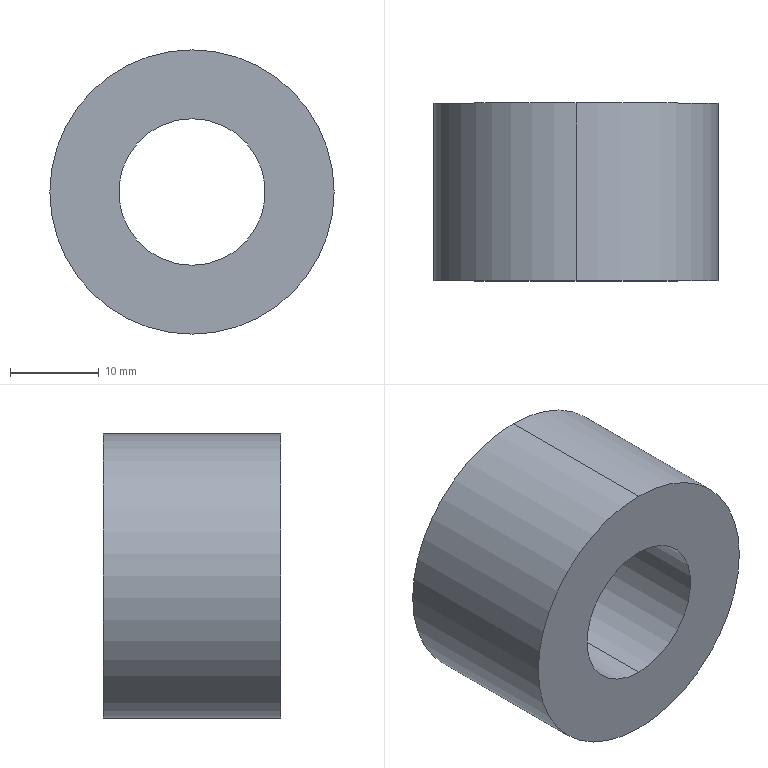Part | SolidWorks | features Chamfer 1, Extrusion 1, HoleWzd 1 | 1 solid | 8 faces | box 32 x 20 x 32 mm | volume 11591 mm3 | cylinder 4 | cone 2 | plane 2 | commonest cylinder face diameters 16.5 x2 32 x2
STEP:
#1=CARTESIAN_POINT('',(0.,17.25,-8.25));
#2=VERTEX_POINT('',#1);
#3=CARTESIAN_POINT('',(0.,17.25,8.25));
#4=VERTEX_POINT('',#3);
#5=CARTESIAN_POINT('',(0.,17.25,0.));
#6=DIRECTION('',(0.,1.,0.));
#7=DIRECTION('',(0.,0.,1.));
#8=AXIS2_PLACEMENT_3D('',#5,#6,#7);
#9=CIRCLE('',#8,8.25);
#10=EDGE_CURVE('',#2,#4,#9,.T.);
#11=ORIENTED_EDGE('',*,*,#10,.F.);
#12=CARTESIAN_POINT('',(0.,20.,-11.));
#13=VERTEX_POINT('',#12);
#14=CARTESIAN_POINT('',(0.,17.25,-8.25));
#15=DIRECTION('',(0.,0.7071,-0.7071));
#16=VECTOR('',#15,1000.);
#17=LINE('',#14,#16);
#18=EDGE_CURVE('',#2,#13,#17,.T.);
#19=ORIENTED_EDGE('',*,*,#18,.T.);
#20=CARTESIAN_POINT('',(0.,20.,11.));
#21=VERTEX_POINT('',#20);
#22=CARTESIAN_POINT('',(0.,20.,0.));
#23=DIRECTION('',(0.,-1.,0.));
#24=DIRECTION('',(0.,0.,1.));
#25=AXIS2_PLACEMENT_3D('',#22,#23,#24);
#26=CIRCLE('',#25,11.);
#27=EDGE_CURVE('',#21,#13,#26,.T.);
#28=ORIENTED_EDGE('',*,*,#27,.F.);
#29=CARTESIAN_POINT('',(0.,17.25,8.25));
#30=DIRECTION('',(0.,0.7071,0.7071));
#31=VECTOR('',#30,1000.);
#32=LINE('',#29,#31);
#33=EDGE_CURVE('',#4,#21,#32,.T.);
#34=ORIENTED_EDGE('',*,*,#33,.F.);
#35=EDGE_LOOP('',(#11,#19,#28,#34));
#36=FACE_OUTER_BOUND('',#35,.T.);
#37=CARTESIAN_POINT('',(0.,17.25,0.));
#38=DIRECTION('',(0.,1.,0.));
#39=DIRECTION('',(0.,0.,1.));
#40=AXIS2_PLACEMENT_3D('',#37,#38,#39);
#41=CONICAL_SURFACE('',#40,8.25,0.7854);
#42=ADVANCED_FACE('',(#36),#41,.F.);
#43=CARTESIAN_POINT('',(0.,0.,-8.25));
#44=VERTEX_POINT('',#43);
#45=CARTESIAN_POINT('',(0.,0.,8.25));
#46=VERTEX_POINT('',#45);
#47=CARTESIAN_POINT('',(0.,0.,0.));
#48=DIRECTION('',(0.,1.,0.));
#49=DIRECTION('',(0.,0.,1.));
#50=AXIS2_PLACEMENT_3D('',#47,#48,#49);
#51=CIRCLE('',#50,8.25);
#52=EDGE_CURVE('',#44,#46,#51,.T.);
#53=ORIENTED_EDGE('',*,*,#52,.F.);
#54=CARTESIAN_POINT('',(0.,20.,-8.25));
#55=DIRECTION('',(0.,1.,0.));
#56=VECTOR('',#55,1000.);
#57=LINE('',#54,#56);
#58=EDGE_CURVE('',#44,#2,#57,.T.);
#59=ORIENTED_EDGE('',*,*,#58,.T.);
#60=ORIENTED_EDGE('',*,*,#10,.T.);
#61=CARTESIAN_POINT('',(0.,20.,8.25));
#62=DIRECTION('',(0.,1.,0.));
#63=VECTOR('',#62,1000.);
#64=LINE('',#61,#63);
#65=EDGE_CURVE('',#46,#4,#64,.T.);
#66=ORIENTED_EDGE('',*,*,#65,.F.);
#67=EDGE_LOOP('',(#53,#59,#60,#66));
#68=FACE_OUTER_BOUND('',#67,.T.);
#69=CARTESIAN_POINT('',(0.,20.,0.));
#70=DIRECTION('',(0.,1.,0.));
#71=DIRECTION('',(0.,0.,1.));
#72=AXIS2_PLACEMENT_3D('',#69,#70,#71);
#73=CYLINDRICAL_SURFACE('',#72,8.25);
#74=ADVANCED_FACE('',(#68),#73,.F.);
#75=CARTESIAN_POINT('',(0.,20.,16.));
#76=VERTEX_POINT('',#75);
#77=CARTESIAN_POINT('',(0.,20.,-16.));
#78=VERTEX_POINT('',#77);
#79=CARTESIAN_POINT('',(0.,20.,0.));
#80=DIRECTION('',(0.,1.,0.));
#81=DIRECTION('',(0.,0.,1.));
#82=AXIS2_PLACEMENT_3D('',#79,#80,#81);
#83=CIRCLE('',#82,16.);
#84=EDGE_CURVE('',#76,#78,#83,.T.);
#85=ORIENTED_EDGE('',*,*,#84,.F.);
#86=CARTESIAN_POINT('',(0.,0.,16.));
#87=VERTEX_POINT('',#86);
#88=CARTESIAN_POINT('',(0.,20.,16.));
#89=DIRECTION('',(0.,-1.,0.));
#90=VECTOR('',#89,1000.);
#91=LINE('',#88,#90);
#92=EDGE_CURVE('',#76,#87,#91,.T.);
#93=ORIENTED_EDGE('',*,*,#92,.T.);
#94=CARTESIAN_POINT('',(0.,0.,-16.));
#95=VERTEX_POINT('',#94);
#96=CARTESIAN_POINT('',(0.,0.,0.));
#97=DIRECTION('',(0.,1.,0.));
#98=DIRECTION('',(0.,0.,1.));
#99=AXIS2_PLACEMENT_3D('',#96,#97,#98);
#100=CIRCLE('',#99,16.);
#101=EDGE_CURVE('',#87,#95,#100,.T.);
#102=ORIENTED_EDGE('',*,*,#101,.T.);
#103=CARTESIAN_POINT('',(0.,20.,-16.));
#104=DIRECTION('',(0.,-1.,0.));
#105=VECTOR('',#104,1000.);
#106=LINE('',#103,#105);
#107=EDGE_CURVE('',#78,#95,#106,.T.);
#108=ORIENTED_EDGE('',*,*,#107,.F.);
#109=EDGE_LOOP('',(#85,#93,#102,#108));
#110=FACE_OUTER_BOUND('',#109,.T.);
#111=CARTESIAN_POINT('',(0.,20.,0.));
#112=DIRECTION('',(0.,-1.,0.));
#113=DIRECTION('',(0.,0.,-1.));
#114=AXIS2_PLACEMENT_3D('',#111,#112,#113);
#115=CYLINDRICAL_SURFACE('',#114,16.);
#116=ADVANCED_FACE('',(#110),#115,.T.);
#117=ORIENTED_EDGE('',*,*,#27,.T.);
#118=CARTESIAN_POINT('',(0.,20.,0.));
#119=DIRECTION('',(0.,-1.,0.));
#120=DIRECTION('',(0.,0.,1.));
#121=AXIS2_PLACEMENT_3D('',#118,#119,#120);
#122=CIRCLE('',#121,11.);
#123=EDGE_CURVE('',#13,#21,#122,.T.);
#124=ORIENTED_EDGE('',*,*,#123,.T.);
#125=EDGE_LOOP('',(#117,#124));
#126=FACE_BOUND('',#125,.T.);
#127=CARTESIAN_POINT('',(0.,20.,0.));
#128=DIRECTION('',(0.,1.,0.));
#129=DIRECTION('',(0.,0.,1.));
#130=AXIS2_PLACEMENT_3D('',#127,#128,#129);
#131=CIRCLE('',#130,16.);
#132=EDGE_CURVE('',#78,#76,#131,.T.);
#133=ORIENTED_EDGE('',*,*,#132,.T.);
#134=ORIENTED_EDGE('',*,*,#84,.T.);
#135=EDGE_LOOP('',(#133,#134));
#136=FACE_OUTER_BOUND('',#135,.T.);
#137=CARTESIAN_POINT('',(0.,20.,0.));
#138=DIRECTION('',(0.,1.,0.));
#139=DIRECTION('',(0.,0.,1.));
#140=AXIS2_PLACEMENT_3D('',#137,#138,#139);
#141=PLANE('',#140);
#142=ADVANCED_FACE('',(#126,#136),#141,.T.);
#143=CARTESIAN_POINT('',(0.,0.,0.));
#144=DIRECTION('',(0.,1.,0.));
#145=DIRECTION('',(0.,0.,1.));
#146=AXIS2_PLACEMENT_3D('',#143,#144,#145);
#147=CIRCLE('',#146,8.25);
#148=EDGE_CURVE('',#46,#44,#147,.T.);
#149=ORIENTED_EDGE('',*,*,#148,.T.);
#150=ORIENTED_EDGE('',*,*,#52,.T.);
#151=EDGE_LOOP('',(#149,#150));
#152=FACE_BOUND('',#151,.T.);
#153=CARTESIAN_POINT('',(0.,0.,0.));
#154=DIRECTION('',(0.,1.,0.));
#155=DIRECTION('',(0.,0.,1.));
#156=AXIS2_PLACEMENT_3D('',#153,#154,#155);
#157=CIRCLE('',#156,16.);
#158=EDGE_CURVE('',#95,#87,#157,.T.);
#159=ORIENTED_EDGE('',*,*,#158,.F.);
#160=ORIENTED_EDGE('',*,*,#101,.F.);
#161=EDGE_LOOP('',(#159,#160));
#162=FACE_OUTER_BOUND('',#161,.T.);
#163=CARTESIAN_POINT('',(0.,0.,0.));
#164=DIRECTION('',(0.,1.,0.));
#165=DIRECTION('',(0.,0.,1.));
#166=AXIS2_PLACEMENT_3D('',#163,#164,#165);
#167=PLANE('',#166);
#168=ADVANCED_FACE('',(#152,#162),#167,.F.);
#169=ORIENTED_EDGE('',*,*,#92,.F.);
#170=ORIENTED_EDGE('',*,*,#132,.F.);
#171=ORIENTED_EDGE('',*,*,#107,.T.);
#172=ORIENTED_EDGE('',*,*,#158,.T.);
#173=EDGE_LOOP('',(#169,#170,#171,#172));
#174=FACE_OUTER_BOUND('',#173,.T.);
#175=CARTESIAN_POINT('',(0.,20.,0.));
#176=DIRECTION('',(0.,-1.,0.));
#177=DIRECTION('',(0.,0.,-1.));
#178=AXIS2_PLACEMENT_3D('',#175,#176,#177);
#179=CYLINDRICAL_SURFACE('',#178,16.);
#180=ADVANCED_FACE('',(#174),#179,.T.);
#181=ORIENTED_EDGE('',*,*,#58,.F.);
#182=ORIENTED_EDGE('',*,*,#148,.F.);
#183=ORIENTED_EDGE('',*,*,#65,.T.);
#184=CARTESIAN_POINT('',(0.,17.25,0.));
#185=DIRECTION('',(0.,1.,0.));
#186=DIRECTION('',(0.,0.,1.));
#187=AXIS2_PLACEMENT_3D('',#184,#185,#186);
#188=CIRCLE('',#187,8.25);
#189=EDGE_CURVE('',#4,#2,#188,.T.);
#190=ORIENTED_EDGE('',*,*,#189,.T.);
#191=EDGE_LOOP('',(#181,#182,#183,#190));
#192=FACE_OUTER_BOUND('',#191,.T.);
#193=CARTESIAN_POINT('',(0.,20.,0.));
#194=DIRECTION('',(0.,1.,0.));
#195=DIRECTION('',(0.,0.,1.));
#196=AXIS2_PLACEMENT_3D('',#193,#194,#195);
#197=CYLINDRICAL_SURFACE('',#196,8.25);
#198=ADVANCED_FACE('',(#192),#197,.F.);
#199=ORIENTED_EDGE('',*,*,#18,.F.);
#200=ORIENTED_EDGE('',*,*,#189,.F.);
#201=ORIENTED_EDGE('',*,*,#33,.T.);
#202=ORIENTED_EDGE('',*,*,#123,.F.);
#203=EDGE_LOOP('',(#199,#200,#201,#202));
#204=FACE_OUTER_BOUND('',#203,.T.);
#205=CARTESIAN_POINT('',(0.,17.25,0.));
#206=DIRECTION('',(0.,1.,0.));
#207=DIRECTION('',(0.,0.,1.));
#208=AXIS2_PLACEMENT_3D('',#205,#206,#207);
#209=CONICAL_SURFACE('',#208,8.25,0.7854);
#210=ADVANCED_FACE('',(#204),#209,.F.);
#211=CLOSED_SHELL('',(#42,#74,#116,#142,#168,#180,#198,#210));
#212=MANIFOLD_SOLID_BREP('',#211);
#213=CARTESIAN_POINT('',(0.,0.,0.));
#214=DIRECTION('',(0.,0.,1.));
#215=DIRECTION('',(1.,0.,0.));
#216=AXIS2_PLACEMENT_3D('',#213,#214,#215);
#217=(LENGTH_UNIT()NAMED_UNIT(*)SI_UNIT(.MILLI.,.METRE.));
#218=UNCERTAINTY_MEASURE_WITH_UNIT(LENGTH_MEASURE(0.00001),#217,'','');
#219=(NAMED_UNIT(*)PLANE_ANGLE_UNIT()SI_UNIT($,.RADIAN.));
#220=(NAMED_UNIT(*)SI_UNIT($,.STERADIAN.)SOLID_ANGLE_UNIT());
#221=(GEOMETRIC_REPRESENTATION_CONTEXT(3)GLOBAL_UNCERTAINTY_ASSIGNED_CONTEXT((#218))GLOBAL_UNIT_ASSIGNED_CONTEXT((#217,#219,#220))REPRESENTATION_CONTEXT('',''));
#222=ADVANCED_BREP_SHAPE_REPRESENTATION('',(#212,#216),#221);